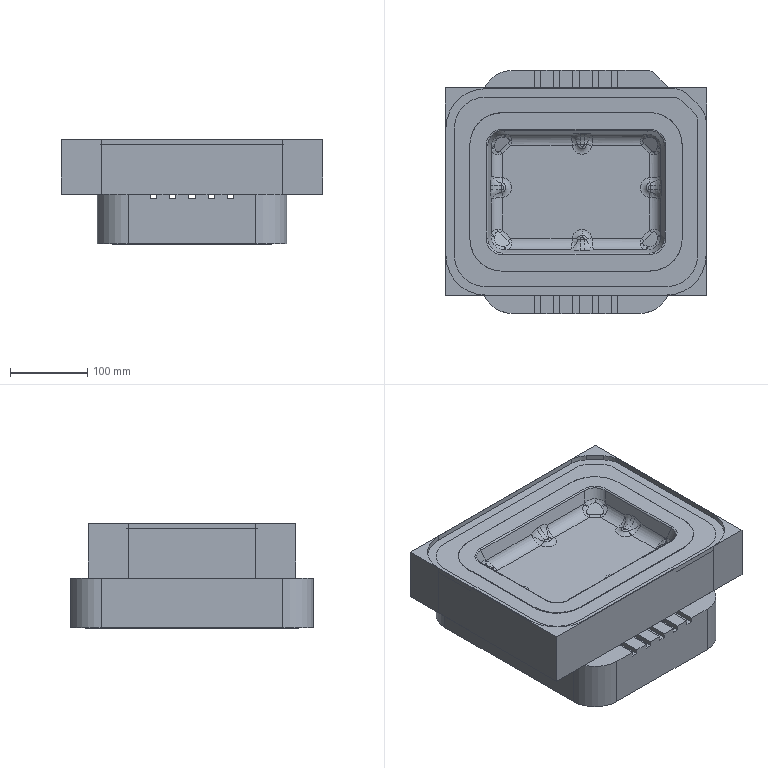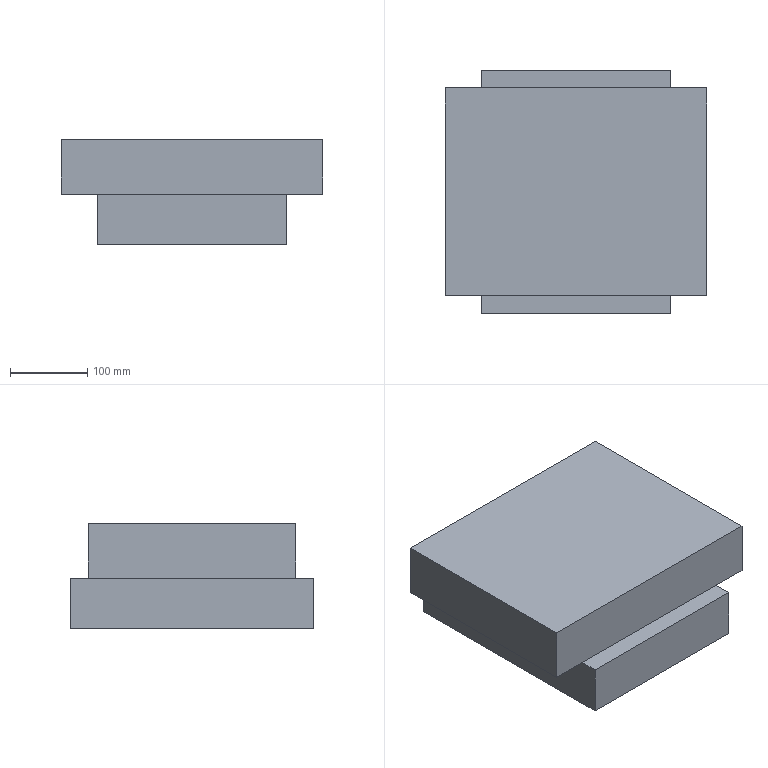CAM job | NX | 3-axis milling, drilling | part box 339.125 x 315.125 x 135.5 mm | stock box 339.125 x 315.125 x 135.5 mm
Tools:
number,name,description,diameter,corner_radius,flute_length,length,flutes
0,V2.0,Drilling Tool,2.0,0.0,35.0,50.0,2
0,V8.0,Drilling Tool,8.0,0.0,35.0,50.0,2
0,D10,No Description,10.0,0.0,20.0,60.0,2
0,D8,No Description,8.0,0.0,0.0,40.0,2
0,D16R0.8,No Description,16.0,0.8,50.0,90.0,2
0,R2,No Description,4.0,2.0,0.0,20.0,2
Operations:
program,operation,operation_type,tool,method,geometry_group,spindle_rpm,surface_speed,feed_per_tooth,feed_cut,feed_plunge,cut_length_mm,path_length_mm,cut_time_min,machine_time_min
B-1,B1,CavityMilling,D16R0.8,METHOD,22B,7000.0,1099.0,0.3214,4500.0,100.0,321938.118,328701.629,71.542,72.218
B-2,B5,SurfaceContour,R2,METHOD,22B,8000.0,251.0,0.2812,4500.0,100.0,237867.201,238614.6,52.859,52.934
B-2,B4,Engraving,R2,METHOD,22B,9000.0,113.0,0.1111,2000.0,100.0,646.755,6659.27,0.6027,1.204
B-3,DRILLING,Operation,V2.0,METHOD,22B,2000.0,75.0,0.0375,150.0,0.0,325.0,2864.565,2.167,2.421
B-4,B6,FaceMilling,D10,METHOD,22B,7000.0,1099.0,0.2857,4000.0,100.0,6030.836,6340.836,1.508,1.539
B-4,B7,PlanarMilling,D10,METHOD,22B,7000.0,571.0,0.2857,4000.0,100.0,75306.928,75681.698,18.827,18.864
C-1,CAVITY_MILL,CavityMilling,D8,METHOD,23C,7000.0,1099.0,0.3214,4500.0,100.0,112294.879,133871.691,24.954,27.112
C-2,DRILLING_1,Operation,V2.0,METHOD,23C,2000.0,75.0,0.0375,150.0,0.0,325.0,2834.832,2.167,2.418
C-3,DRILLING_1_COPY,Operation,V8.0,METHOD,23C,2000.0,75.0,0.0375,150.0,0.0,1260.0,3670.747,8.4,8.641
C-3,DRILLING_1_COPY_COPY,Operation,V8.0,METHOD,23C,2000.0,75.0,0.0375,150.0,0.0,420.0,2127.983,2.8,2.971